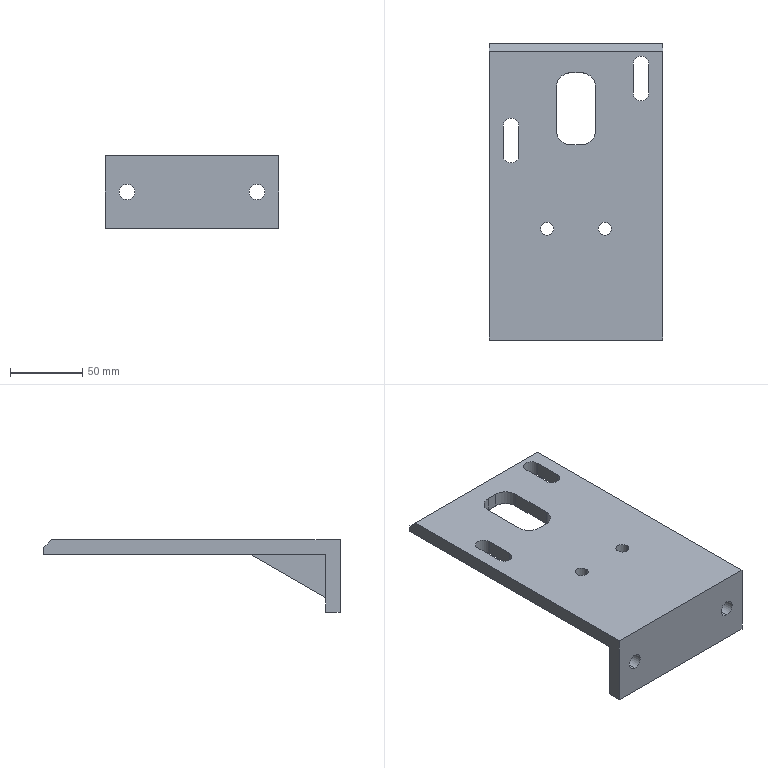NC program | NX | posted with a generic post | part box 120 x 205 x 50 mm
Lines 7099 to 7208 of 11006:
(ZLEVEL_PROFILE_COPY_1_COPY_COPY_1_COPY_1 , TOOL : D10JING)
N14196 T14 M6
N14198 G54
N14200 G17 G0 G90 X-85.625 Y66.858 B0. C0. S9500 M3
N14202 G43 Z30. H14
N14204 Z-8.9
N14206 G94 G1 Z-9.9 F1000.
N14208 X-87.007 Y66.048
N14210 G3 X-87.501 Y65.179 R1.
N14212 G1 X-87.498 Y64.793 F1200.
N14214 X-87.5 Y59.393
N14216 Y-60.
N14218 X-87.504 Y-60.188
N14220 X-87.503 Y-65.179
N14222 G3 X-87.003 Y-66.045 R1.
N14224 G1 X-85.624 Y-66.841
N14226 Z-8.9
N14228 G0 Z30.
(ZLEVEL_PROFILE_COPY_1_COPY_COPY_1_COPY_1_COPY , TOOL : D10JING)
N14230 X-53.908 Y8.197
N14232 Z-24.
N14234 G1 Z-25. F1000.
N14236 X-54.661 Y9.5
N14238 G3 X-55.527 Y10. R1.
N14240 G1 X-87.5 F1200.
N14242 Y-10.
N14244 X-55.527
N14246 G3 X-54.661 Y-9.5 R1.
N14248 G1 X-53.904 Y-8.189
N14250 Z-24.
N14252 G0 Z30.
N14254 X-33.284 Y8.1
N14256 Z-39.
N14258 G1 Z-40. F1000.
N14260 X-34.091 Y9.5
N14262 G3 X-34.957 Y10. R1.
N14264 G1 X-40.551 F1200.
N14266 X-87.5
N14268 Y-10.
N14270 X-40.551
N14272 X-34.957
N14274 G3 X-34.091 Y-9.5 R1.
N14276 G1 X-33.279 Y-8.091
N14278 Z-39.
N14280 G0 Z30.
N14282 X-53.993 Y-31.834
N14284 Z-24.
N14286 G1 Z-25. F1000.
N14288 X-54.763 Y-30.5
N14290 G3 X-55.629 Y-30. R1.
N14292 G1 X-87.5 F1200.
N14294 Y-60.
N14296 X-87.562 Y-60.783
N14298 X-87.5 Y-60.777
N14300 X-87.501 Y-60.84
N14302 X-87.502 Y-65.179
N14304 G3 X-87.002 Y-66.045 R1.
N14306 G1 X-85.623 Y-66.841
N14308 Z-24.
N14310 G0 Z30.
N14312 X-33.286 Y-31.895
N14314 Z-39.
N14316 G1 Z-40. F1000.
N14318 X-34.091 Y-30.5
N14320 G3 X-34.957 Y-30. R1.
N14322 G1 X-40.551 F1200.
N14324 X-87.5
N14326 Y-60.019
N14328 G2 X-87.554 Y-60.736 R4.75
N14330 G1 X-87.496 Y-60.733
N14332 X-87.499 Y-60.792
N14334 X-87.5 Y-65.179
N14336 G3 X-87. Y-66.045 R1.
N14338 G1 X-85.621 Y-66.841
N14340 Z-39.
N14342 G0 Z30.
N14344 X-85.624 Y66.86
N14346 Z-24.
N14348 G1 Z-25. F1000.
N14350 X-87.006 Y66.048
N14352 G3 X-87.499 Y65.179 R1.
N14354 G1 X-87.496 Y64.793 F1200.
N14356 Y60.165
N14358 X-87.5 Y60.
N14360 Y30.
N14362 X-55.629
N14364 G3 X-54.763 Y30.5 R1.
N14366 G1 X-53.993 Y31.834
N14368 Z-24.
N14370 G0 Z30.
N14372 X-85.623 Y66.863
N14374 Z-39.
N14376 G1 Z-40. F1000.
N14378 X-87.005 Y66.049
N14380 G3 X-87.497 Y65.179 R1.
N14382 G1 X-87.494 Y64.793 F1200.
N14384 Y60.165
N14386 X-87.5 Y60.
N14388 Y30.
N14390 X-40.551
N14392 X-34.957
N14394 G3 X-34.091 Y30.5 R1.
N14396 G1 X-33.278 Y31.908
N14398 Z-39.
N14400 G0 Z30.
N14402 M5